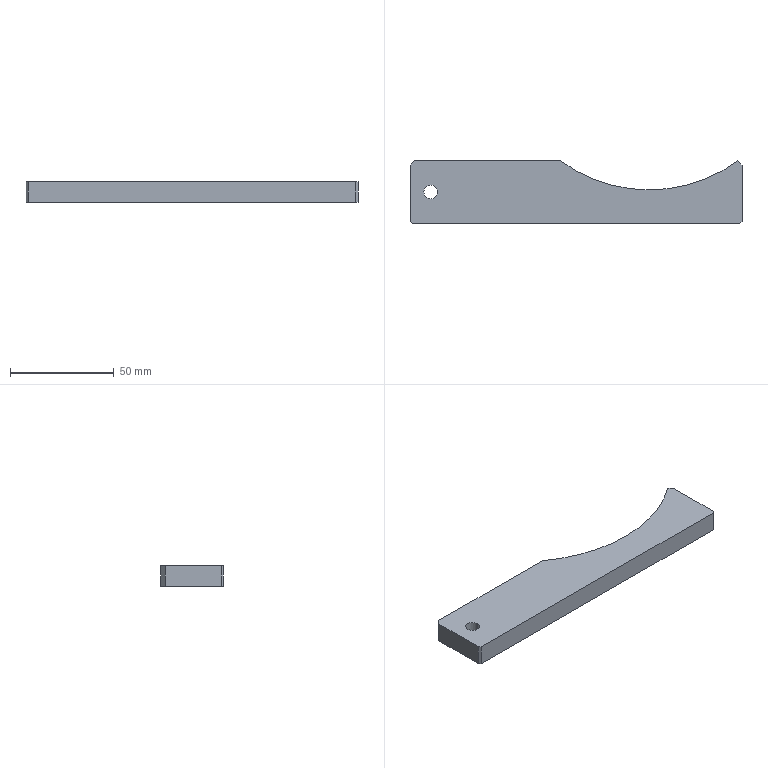Part | SolidWorks | features Chamfer 2, Extrusion 1, HoleWzd 1, ICE 1 | 1 solid | 13 faces | box 160 x 30 x 10 mm | volume 39472 mm3 | plane 10 | cylinder 3 | commonest cylinder face diameters 6.6 x2 144.586 x1
STEP:
#1=CARTESIAN_POINT('',(-73.3,0.,0.));
#2=VERTEX_POINT('',#1);
#3=CARTESIAN_POINT('',(-66.7,0.,0.));
#4=VERTEX_POINT('',#3);
#5=CARTESIAN_POINT('',(-70.,0.,0.));
#6=DIRECTION('',(0.,0.,1.));
#7=DIRECTION('',(1.,0.,0.));
#8=AXIS2_PLACEMENT_3D('',#5,#6,#7);
#9=CIRCLE('',#8,3.3);
#10=EDGE_CURVE('',#2,#4,#9,.T.);
#11=ORIENTED_EDGE('',*,*,#10,.F.);
#12=CARTESIAN_POINT('',(-73.3,0.,10.));
#13=VERTEX_POINT('',#12);
#14=CARTESIAN_POINT('',(-73.3,0.,10.));
#15=DIRECTION('',(0.,0.,1.));
#16=VECTOR('',#15,1000.);
#17=LINE('',#14,#16);
#18=EDGE_CURVE('',#2,#13,#17,.T.);
#19=ORIENTED_EDGE('',*,*,#18,.T.);
#20=CARTESIAN_POINT('',(-66.7,0.,10.));
#21=VERTEX_POINT('',#20);
#22=CARTESIAN_POINT('',(-70.,0.,10.));
#23=DIRECTION('',(0.,0.,1.));
#24=DIRECTION('',(1.,0.,0.));
#25=AXIS2_PLACEMENT_3D('',#22,#23,#24);
#26=CIRCLE('',#25,3.3);
#27=EDGE_CURVE('',#13,#21,#26,.T.);
#28=ORIENTED_EDGE('',*,*,#27,.T.);
#29=CARTESIAN_POINT('',(-66.7,0.,10.));
#30=DIRECTION('',(0.,0.,1.));
#31=VECTOR('',#30,1000.);
#32=LINE('',#29,#31);
#33=EDGE_CURVE('',#4,#21,#32,.T.);
#34=ORIENTED_EDGE('',*,*,#33,.F.);
#35=EDGE_LOOP('',(#11,#19,#28,#34));
#36=FACE_OUTER_BOUND('',#35,.T.);
#37=CARTESIAN_POINT('',(-70.,0.,10.));
#38=DIRECTION('',(0.,0.,1.));
#39=DIRECTION('',(1.,0.,0.));
#40=AXIS2_PLACEMENT_3D('',#37,#38,#39);
#41=CYLINDRICAL_SURFACE('',#40,3.3);
#42=ADVANCED_FACE('',(#36),#41,.F.);
#43=CARTESIAN_POINT('',(80.,-14.,10.));
#44=VERTEX_POINT('',#43);
#45=CARTESIAN_POINT('',(80.,13.,10.));
#46=VERTEX_POINT('',#45);
#47=CARTESIAN_POINT('',(80.,-15.,10.));
#48=DIRECTION('',(0.,1.,0.));
#49=VECTOR('',#48,1000.);
#50=LINE('',#47,#49);
#51=EDGE_CURVE('',#44,#46,#50,.T.);
#52=ORIENTED_EDGE('',*,*,#51,.F.);
#53=CARTESIAN_POINT('',(80.,-14.,0.));
#54=VERTEX_POINT('',#53);
#55=CARTESIAN_POINT('',(80.,-14.,10.));
#56=DIRECTION('',(0.,0.,-1.));
#57=VECTOR('',#56,1000.);
#58=LINE('',#55,#57);
#59=EDGE_CURVE('',#44,#54,#58,.T.);
#60=ORIENTED_EDGE('',*,*,#59,.T.);
#61=CARTESIAN_POINT('',(80.,13.,0.));
#62=VERTEX_POINT('',#61);
#63=CARTESIAN_POINT('',(80.,-15.,0.));
#64=DIRECTION('',(0.,1.,0.));
#65=VECTOR('',#64,1000.);
#66=LINE('',#63,#65);
#67=EDGE_CURVE('',#54,#62,#66,.T.);
#68=ORIENTED_EDGE('',*,*,#67,.T.);
#69=CARTESIAN_POINT('',(80.,13.,10.));
#70=DIRECTION('',(0.,0.,1.));
#71=VECTOR('',#70,1000.);
#72=LINE('',#69,#71);
#73=EDGE_CURVE('',#62,#46,#72,.T.);
#74=ORIENTED_EDGE('',*,*,#73,.T.);
#75=EDGE_LOOP('',(#52,#60,#68,#74));
#76=FACE_OUTER_BOUND('',#75,.T.);
#77=CARTESIAN_POINT('',(80.,-15.,10.));
#78=DIRECTION('',(-1.,0.,0.));
#79=DIRECTION('',(0.,0.,1.));
#80=AXIS2_PLACEMENT_3D('',#77,#78,#79);
#81=PLANE('',#80);
#82=ADVANCED_FACE('',(#76),#81,.F.);
#83=CARTESIAN_POINT('',(-7.468,15.,10.));
#84=VERTEX_POINT('',#83);
#85=CARTESIAN_POINT('',(-78.,15.,10.));
#86=VERTEX_POINT('',#85);
#87=CARTESIAN_POINT('',(-80.,15.,10.));
#88=DIRECTION('',(-1.,0.,0.));
#89=VECTOR('',#88,1000.);
#90=LINE('',#87,#89);
#91=EDGE_CURVE('',#84,#86,#90,.T.);
#92=ORIENTED_EDGE('',*,*,#91,.F.);
#93=CARTESIAN_POINT('',(-7.468,15.,0.));
#94=VERTEX_POINT('',#93);
#95=CARTESIAN_POINT('',(-7.468,15.,0.));
#96=DIRECTION('',(0.,0.,1.));
#97=VECTOR('',#96,1000.);
#98=LINE('',#95,#97);
#99=EDGE_CURVE('',#94,#84,#98,.T.);
#100=ORIENTED_EDGE('',*,*,#99,.F.);
#101=CARTESIAN_POINT('',(-78.,15.,0.));
#102=VERTEX_POINT('',#101);
#103=CARTESIAN_POINT('',(-80.,15.,0.));
#104=DIRECTION('',(-1.,0.,0.));
#105=VECTOR('',#104,1000.);
#106=LINE('',#103,#105);
#107=EDGE_CURVE('',#94,#102,#106,.T.);
#108=ORIENTED_EDGE('',*,*,#107,.T.);
#109=CARTESIAN_POINT('',(-78.,15.,10.));
#110=DIRECTION('',(0.,0.,1.));
#111=VECTOR('',#110,1000.);
#112=LINE('',#109,#111);
#113=EDGE_CURVE('',#102,#86,#112,.T.);
#114=ORIENTED_EDGE('',*,*,#113,.T.);
#115=EDGE_LOOP('',(#92,#100,#108,#114));
#116=FACE_OUTER_BOUND('',#115,.T.);
#117=CARTESIAN_POINT('',(-80.,15.,10.));
#118=DIRECTION('',(0.,-1.,0.));
#119=DIRECTION('',(0.,0.,-1.));
#120=AXIS2_PLACEMENT_3D('',#117,#118,#119);
#121=PLANE('',#120);
#122=ADVANCED_FACE('',(#116),#121,.F.);
#123=CARTESIAN_POINT('',(-80.,13.,0.));
#124=VERTEX_POINT('',#123);
#125=CARTESIAN_POINT('',(-80.,-14.,0.));
#126=VERTEX_POINT('',#125);
#127=CARTESIAN_POINT('',(-80.,-15.,0.));
#128=DIRECTION('',(0.,-1.,0.));
#129=VECTOR('',#128,1000.);
#130=LINE('',#127,#129);
#131=EDGE_CURVE('',#124,#126,#130,.T.);
#132=ORIENTED_EDGE('',*,*,#131,.T.);
#133=CARTESIAN_POINT('',(-80.,-14.,10.));
#134=VERTEX_POINT('',#133);
#135=CARTESIAN_POINT('',(-80.,-14.,10.));
#136=DIRECTION('',(0.,0.,1.));
#137=VECTOR('',#136,1000.);
#138=LINE('',#135,#137);
#139=EDGE_CURVE('',#126,#134,#138,.T.);
#140=ORIENTED_EDGE('',*,*,#139,.T.);
#141=CARTESIAN_POINT('',(-80.,13.,10.));
#142=VERTEX_POINT('',#141);
#143=CARTESIAN_POINT('',(-80.,-15.,10.));
#144=DIRECTION('',(0.,-1.,0.));
#145=VECTOR('',#144,1000.);
#146=LINE('',#143,#145);
#147=EDGE_CURVE('',#142,#134,#146,.T.);
#148=ORIENTED_EDGE('',*,*,#147,.F.);
#149=CARTESIAN_POINT('',(-80.,13.,10.));
#150=DIRECTION('',(0.,0.,-1.));
#151=VECTOR('',#150,1000.);
#152=LINE('',#149,#151);
#153=EDGE_CURVE('',#142,#124,#152,.T.);
#154=ORIENTED_EDGE('',*,*,#153,.T.);
#155=EDGE_LOOP('',(#132,#140,#148,#154));
#156=FACE_OUTER_BOUND('',#155,.T.);
#157=CARTESIAN_POINT('',(-80.,-15.,10.));
#158=DIRECTION('',(1.,0.,0.));
#159=DIRECTION('',(0.,0.,-1.));
#160=AXIS2_PLACEMENT_3D('',#157,#158,#159);
#161=PLANE('',#160);
#162=ADVANCED_FACE('',(#156),#161,.F.);
#163=CARTESIAN_POINT('',(-79.,-15.,10.));
#164=VERTEX_POINT('',#163);
#165=CARTESIAN_POINT('',(79.,-15.,10.));
#166=VERTEX_POINT('',#165);
#167=CARTESIAN_POINT('',(-80.,-15.,10.));
#168=DIRECTION('',(1.,0.,0.));
#169=VECTOR('',#168,1000.);
#170=LINE('',#167,#169);
#171=EDGE_CURVE('',#164,#166,#170,.T.);
#172=ORIENTED_EDGE('',*,*,#171,.F.);
#173=CARTESIAN_POINT('',(-79.,-15.,0.));
#174=VERTEX_POINT('',#173);
#175=CARTESIAN_POINT('',(-79.,-15.,10.));
#176=DIRECTION('',(0.,0.,-1.));
#177=VECTOR('',#176,1000.);
#178=LINE('',#175,#177);
#179=EDGE_CURVE('',#164,#174,#178,.T.);
#180=ORIENTED_EDGE('',*,*,#179,.T.);
#181=CARTESIAN_POINT('',(79.,-15.,0.));
#182=VERTEX_POINT('',#181);
#183=CARTESIAN_POINT('',(-80.,-15.,0.));
#184=DIRECTION('',(1.,0.,0.));
#185=VECTOR('',#184,1000.);
#186=LINE('',#183,#185);
#187=EDGE_CURVE('',#174,#182,#186,.T.);
#188=ORIENTED_EDGE('',*,*,#187,.T.);
#189=CARTESIAN_POINT('',(79.,-15.,10.));
#190=DIRECTION('',(0.,0.,1.));
#191=VECTOR('',#190,1000.);
#192=LINE('',#189,#191);
#193=EDGE_CURVE('',#182,#166,#192,.T.);
#194=ORIENTED_EDGE('',*,*,#193,.T.);
#195=EDGE_LOOP('',(#172,#180,#188,#194));
#196=FACE_OUTER_BOUND('',#195,.T.);
#197=CARTESIAN_POINT('',(-80.,-15.,10.));
#198=DIRECTION('',(0.,1.,0.));
#199=DIRECTION('',(0.,0.,1.));
#200=AXIS2_PLACEMENT_3D('',#197,#198,#199);
#201=PLANE('',#200);
#202=ADVANCED_FACE('',(#196),#201,.F.);
#203=CARTESIAN_POINT('',(-70.,0.,10.));
#204=DIRECTION('',(0.,0.,1.));
#205=DIRECTION('',(1.,0.,0.));
#206=AXIS2_PLACEMENT_3D('',#203,#204,#205);
#207=CIRCLE('',#206,3.3);
#208=EDGE_CURVE('',#21,#13,#207,.T.);
#209=ORIENTED_EDGE('',*,*,#208,.F.);
#210=ORIENTED_EDGE('',*,*,#27,.F.);
#211=EDGE_LOOP('',(#209,#210));
#212=FACE_BOUND('',#211,.T.);
#213=CARTESIAN_POINT('',(78.,15.,10.));
#214=VERTEX_POINT('',#213);
#215=CARTESIAN_POINT('',(78.,15.,10.));
#216=DIRECTION('',(-0.7071,0.7071,0.));
#217=VECTOR('',#216,1000.);
#218=LINE('',#215,#217);
#219=EDGE_CURVE('',#46,#214,#218,.T.);
#220=ORIENTED_EDGE('',*,*,#219,.T.);
#221=CARTESIAN_POINT('',(35.266,73.31,10.));
#222=DIRECTION('',(0.,0.,1.));
#223=DIRECTION('',(-1.,0.,0.));
#224=AXIS2_PLACEMENT_3D('',#221,#222,#223);
#225=CIRCLE('',#224,72.293);
#226=EDGE_CURVE('',#84,#214,#225,.T.);
#227=ORIENTED_EDGE('',*,*,#226,.F.);
#228=ORIENTED_EDGE('',*,*,#91,.T.);
#229=CARTESIAN_POINT('',(-80.,13.,10.));
#230=DIRECTION('',(-0.7071,-0.7071,0.));
#231=VECTOR('',#230,1000.);
#232=LINE('',#229,#231);
#233=EDGE_CURVE('',#86,#142,#232,.T.);
#234=ORIENTED_EDGE('',*,*,#233,.T.);
#235=ORIENTED_EDGE('',*,*,#147,.T.);
#236=CARTESIAN_POINT('',(-79.,-15.,10.));
#237=DIRECTION('',(0.7071,-0.7071,0.));
#238=VECTOR('',#237,1000.);
#239=LINE('',#236,#238);
#240=EDGE_CURVE('',#134,#164,#239,.T.);
#241=ORIENTED_EDGE('',*,*,#240,.T.);
#242=ORIENTED_EDGE('',*,*,#171,.T.);
#243=CARTESIAN_POINT('',(80.,-14.,10.));
#244=DIRECTION('',(0.7071,0.7071,0.));
#245=VECTOR('',#244,1000.);
#246=LINE('',#243,#245);
#247=EDGE_CURVE('',#166,#44,#246,.T.);
#248=ORIENTED_EDGE('',*,*,#247,.T.);
#249=ORIENTED_EDGE('',*,*,#51,.T.);
#250=EDGE_LOOP('',(#220,#227,#228,#234,#235,#241,#242,#248,#249));
#251=FACE_OUTER_BOUND('',#250,.T.);
#252=CARTESIAN_POINT('',(0.,0.,10.));
#253=DIRECTION('',(0.,0.,-1.));
#254=DIRECTION('',(-1.,0.,0.));
#255=AXIS2_PLACEMENT_3D('',#252,#253,#254);
#256=PLANE('',#255);
#257=ADVANCED_FACE('',(#212,#251),#256,.F.);
#258=CARTESIAN_POINT('',(78.,15.,0.));
#259=VERTEX_POINT('',#258);
#260=CARTESIAN_POINT('',(35.266,73.31,0.));
#261=DIRECTION('',(0.,0.,1.));
#262=DIRECTION('',(-1.,0.,0.));
#263=AXIS2_PLACEMENT_3D('',#260,#261,#262);
#264=CIRCLE('',#263,72.293);
#265=EDGE_CURVE('',#94,#259,#264,.T.);
#266=ORIENTED_EDGE('',*,*,#265,.T.);
#267=CARTESIAN_POINT('',(46.5,46.5,0.));
#268=DIRECTION('',(0.7071,-0.7071,0.));
#269=VECTOR('',#268,1000.);
#270=LINE('',#267,#269);
#271=EDGE_CURVE('',#259,#62,#270,.T.);
#272=ORIENTED_EDGE('',*,*,#271,.T.);
#273=ORIENTED_EDGE('',*,*,#67,.F.);
#274=CARTESIAN_POINT('',(47.,-47.,0.));
#275=DIRECTION('',(-0.7071,-0.7071,0.));
#276=VECTOR('',#275,1000.);
#277=LINE('',#274,#276);
#278=EDGE_CURVE('',#54,#182,#277,.T.);
#279=ORIENTED_EDGE('',*,*,#278,.T.);
#280=ORIENTED_EDGE('',*,*,#187,.F.);
#281=CARTESIAN_POINT('',(-47.,-47.,0.));
#282=DIRECTION('',(-0.7071,0.7071,0.));
#283=VECTOR('',#282,1000.);
#284=LINE('',#281,#283);
#285=EDGE_CURVE('',#174,#126,#284,.T.);
#286=ORIENTED_EDGE('',*,*,#285,.T.);
#287=ORIENTED_EDGE('',*,*,#131,.F.);
#288=CARTESIAN_POINT('',(-46.5,46.5,0.));
#289=DIRECTION('',(0.7071,0.7071,0.));
#290=VECTOR('',#289,1000.);
#291=LINE('',#288,#290);
#292=EDGE_CURVE('',#124,#102,#291,.T.);
#293=ORIENTED_EDGE('',*,*,#292,.T.);
#294=ORIENTED_EDGE('',*,*,#107,.F.);
#295=EDGE_LOOP('',(#266,#272,#273,#279,#280,#286,#287,#293,#294));
#296=FACE_OUTER_BOUND('',#295,.T.);
#297=CARTESIAN_POINT('',(-70.,0.,0.));
#298=DIRECTION('',(0.,0.,1.));
#299=DIRECTION('',(1.,0.,0.));
#300=AXIS2_PLACEMENT_3D('',#297,#298,#299);
#301=CIRCLE('',#300,3.3);
#302=EDGE_CURVE('',#4,#2,#301,.T.);
#303=ORIENTED_EDGE('',*,*,#302,.T.);
#304=ORIENTED_EDGE('',*,*,#10,.T.);
#305=EDGE_LOOP('',(#303,#304));
#306=FACE_BOUND('',#305,.T.);
#307=CARTESIAN_POINT('',(0.,0.,0.));
#308=DIRECTION('',(0.,0.,-1.));
#309=DIRECTION('',(-1.,0.,0.));
#310=AXIS2_PLACEMENT_3D('',#307,#308,#309);
#311=PLANE('',#310);
#312=ADVANCED_FACE('',(#296,#306),#311,.T.);
#313=ORIENTED_EDGE('',*,*,#233,.F.);
#314=ORIENTED_EDGE('',*,*,#113,.F.);
#315=ORIENTED_EDGE('',*,*,#292,.F.);
#316=ORIENTED_EDGE('',*,*,#153,.F.);
#317=EDGE_LOOP('',(#313,#314,#315,#316));
#318=FACE_OUTER_BOUND('',#317,.T.);
#319=CARTESIAN_POINT('',(-80.,13.,10.));
#320=DIRECTION('',(0.7071,-0.7071,0.));
#321=DIRECTION('',(0.,0.,-1.));
#322=AXIS2_PLACEMENT_3D('',#319,#320,#321);
#323=PLANE('',#322);
#324=ADVANCED_FACE('',(#318),#323,.F.);
#325=ORIENTED_EDGE('',*,*,#219,.F.);
#326=ORIENTED_EDGE('',*,*,#73,.F.);
#327=ORIENTED_EDGE('',*,*,#271,.F.);
#328=CARTESIAN_POINT('',(78.,15.,10.));
#329=DIRECTION('',(0.,0.,-1.));
#330=VECTOR('',#329,1000.);
#331=LINE('',#328,#330);
#332=EDGE_CURVE('',#214,#259,#331,.T.);
#333=ORIENTED_EDGE('',*,*,#332,.F.);
#334=EDGE_LOOP('',(#325,#326,#327,#333));
#335=FACE_OUTER_BOUND('',#334,.T.);
#336=CARTESIAN_POINT('',(78.,15.,10.));
#337=DIRECTION('',(-0.7071,-0.7071,0.));
#338=DIRECTION('',(0.,0.,-1.));
#339=AXIS2_PLACEMENT_3D('',#336,#337,#338);
#340=PLANE('',#339);
#341=ADVANCED_FACE('',(#335),#340,.F.);
#342=ORIENTED_EDGE('',*,*,#240,.F.);
#343=ORIENTED_EDGE('',*,*,#139,.F.);
#344=ORIENTED_EDGE('',*,*,#285,.F.);
#345=ORIENTED_EDGE('',*,*,#179,.F.);
#346=EDGE_LOOP('',(#342,#343,#344,#345));
#347=FACE_OUTER_BOUND('',#346,.T.);
#348=CARTESIAN_POINT('',(-79.,-15.,10.));
#349=DIRECTION('',(0.7071,0.7071,0.));
#350=DIRECTION('',(0.,0.,-1.));
#351=AXIS2_PLACEMENT_3D('',#348,#349,#350);
#352=PLANE('',#351);
#353=ADVANCED_FACE('',(#347),#352,.F.);
#354=ORIENTED_EDGE('',*,*,#247,.F.);
#355=ORIENTED_EDGE('',*,*,#193,.F.);
#356=ORIENTED_EDGE('',*,*,#278,.F.);
#357=ORIENTED_EDGE('',*,*,#59,.F.);
#358=EDGE_LOOP('',(#354,#355,#356,#357));
#359=FACE_OUTER_BOUND('',#358,.T.);
#360=CARTESIAN_POINT('',(80.,-14.,10.));
#361=DIRECTION('',(-0.7071,0.7071,0.));
#362=DIRECTION('',(0.,0.,-1.));
#363=AXIS2_PLACEMENT_3D('',#360,#361,#362);
#364=PLANE('',#363);
#365=ADVANCED_FACE('',(#359),#364,.F.);
#366=ORIENTED_EDGE('',*,*,#18,.F.);
#367=ORIENTED_EDGE('',*,*,#302,.F.);
#368=ORIENTED_EDGE('',*,*,#33,.T.);
#369=ORIENTED_EDGE('',*,*,#208,.T.);
#370=EDGE_LOOP('',(#366,#367,#368,#369));
#371=FACE_OUTER_BOUND('',#370,.T.);
#372=CARTESIAN_POINT('',(-70.,0.,10.));
#373=DIRECTION('',(0.,0.,1.));
#374=DIRECTION('',(1.,0.,0.));
#375=AXIS2_PLACEMENT_3D('',#372,#373,#374);
#376=CYLINDRICAL_SURFACE('',#375,3.3);
#377=ADVANCED_FACE('',(#371),#376,.F.);
#378=ORIENTED_EDGE('',*,*,#226,.T.);
#379=ORIENTED_EDGE('',*,*,#332,.T.);
#380=ORIENTED_EDGE('',*,*,#265,.F.);
#381=ORIENTED_EDGE('',*,*,#99,.T.);
#382=EDGE_LOOP('',(#378,#379,#380,#381));
#383=FACE_OUTER_BOUND('',#382,.T.);
#384=CARTESIAN_POINT('',(35.266,73.31,0.));
#385=DIRECTION('',(0.,0.,1.));
#386=DIRECTION('',(1.,0.,0.));
#387=AXIS2_PLACEMENT_3D('',#384,#385,#386);
#388=CYLINDRICAL_SURFACE('',#387,72.293);
#389=ADVANCED_FACE('',(#383),#388,.F.);
#390=CLOSED_SHELL('',(#42,#82,#122,#162,#202,#257,#312,#324,#341,#353,#365,#377,#389));
#391=MANIFOLD_SOLID_BREP('',#390);
#392=CARTESIAN_POINT('',(0.,0.,0.));
#393=DIRECTION('',(0.,0.,1.));
#394=DIRECTION('',(1.,0.,0.));
#395=AXIS2_PLACEMENT_3D('',#392,#393,#394);
#396=(LENGTH_UNIT()NAMED_UNIT(*)SI_UNIT(.MILLI.,.METRE.));
#397=UNCERTAINTY_MEASURE_WITH_UNIT(LENGTH_MEASURE(0.00001),#396,'','');
#398=(NAMED_UNIT(*)PLANE_ANGLE_UNIT()SI_UNIT($,.RADIAN.));
#399=(NAMED_UNIT(*)SI_UNIT($,.STERADIAN.)SOLID_ANGLE_UNIT());
#400=(GEOMETRIC_REPRESENTATION_CONTEXT(3)GLOBAL_UNCERTAINTY_ASSIGNED_CONTEXT((#397))GLOBAL_UNIT_ASSIGNED_CONTEXT((#396,#398,#399))REPRESENTATION_CONTEXT('',''));
#401=ADVANCED_BREP_SHAPE_REPRESENTATION('',(#391,#395),#400);